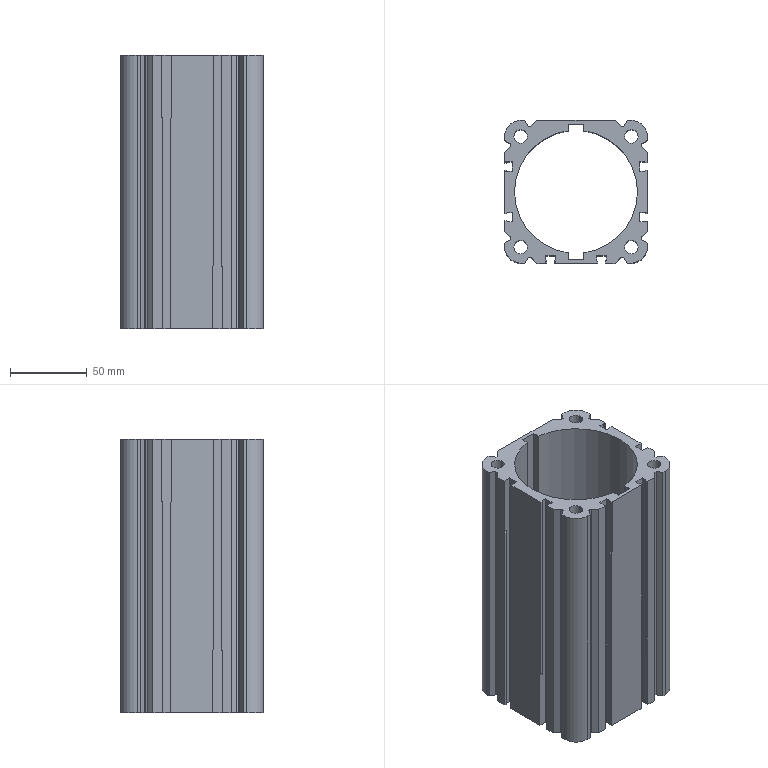Part | SolidWorks | features ICE 6, CirPattern 4, Fillet 3, Extrusion 1, HoleWzd 1 | 1 solid | 129 faces | box 93 x 93 x 178 mm | volume 509573 mm3 | plane 92 | cylinder 37 | commonest cylinder face diameters 4 x12 3 x8 8.7 x8 22 x4 80 x3 9 x2